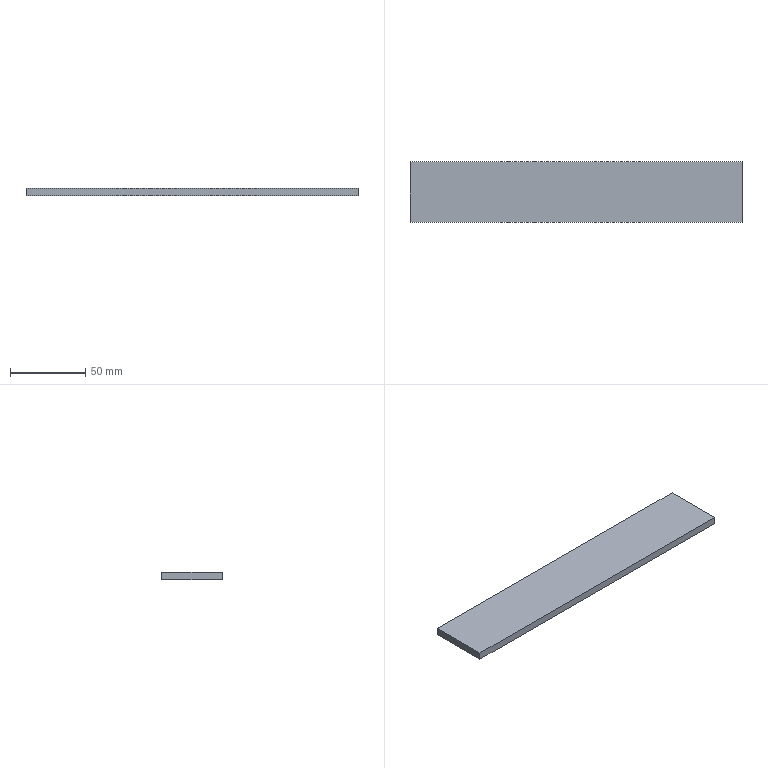Part | SolidWorks | features BaseBody 1 | 1 solid | 6 faces | box 220 x 40 x 5 mm | volume 44000 mm3 | plane 6
STEP:
#1=CARTESIAN_POINT('',(110.,-20.,0.));
#2=VERTEX_POINT('',#1);
#3=CARTESIAN_POINT('',(110.,20.,0.));
#4=VERTEX_POINT('',#3);
#5=CARTESIAN_POINT('',(110.,20.,0.));
#6=DIRECTION('',(0.,1.,0.));
#7=VECTOR('',#6,1000.);
#8=LINE('',#5,#7);
#9=EDGE_CURVE('',#2,#4,#8,.T.);
#10=ORIENTED_EDGE('',*,*,#9,.T.);
#11=CARTESIAN_POINT('',(-110.,20.,0.));
#12=VERTEX_POINT('',#11);
#13=CARTESIAN_POINT('',(-110.,20.,0.));
#14=DIRECTION('',(-1.,0.,0.));
#15=VECTOR('',#14,1000.);
#16=LINE('',#13,#15);
#17=EDGE_CURVE('',#4,#12,#16,.T.);
#18=ORIENTED_EDGE('',*,*,#17,.T.);
#19=CARTESIAN_POINT('',(-110.,-20.,0.));
#20=VERTEX_POINT('',#19);
#21=CARTESIAN_POINT('',(-110.,20.,0.));
#22=DIRECTION('',(0.,-1.,0.));
#23=VECTOR('',#22,1000.);
#24=LINE('',#21,#23);
#25=EDGE_CURVE('',#12,#20,#24,.T.);
#26=ORIENTED_EDGE('',*,*,#25,.T.);
#27=CARTESIAN_POINT('',(-110.,-20.,0.));
#28=DIRECTION('',(1.,0.,0.));
#29=VECTOR('',#28,1000.);
#30=LINE('',#27,#29);
#31=EDGE_CURVE('',#20,#2,#30,.T.);
#32=ORIENTED_EDGE('',*,*,#31,.T.);
#33=EDGE_LOOP('',(#10,#18,#26,#32));
#34=FACE_OUTER_BOUND('',#33,.T.);
#35=CARTESIAN_POINT('',(0.,0.,0.));
#36=DIRECTION('',(0.,0.,1.));
#37=DIRECTION('',(1.,0.,0.));
#38=AXIS2_PLACEMENT_3D('',#35,#36,#37);
#39=PLANE('',#38);
#40=ADVANCED_FACE('',(#34),#39,.T.);
#41=CARTESIAN_POINT('',(110.,-20.,-5.));
#42=VERTEX_POINT('',#41);
#43=CARTESIAN_POINT('',(110.,20.,-5.));
#44=VERTEX_POINT('',#43);
#45=CARTESIAN_POINT('',(110.,20.,-5.));
#46=DIRECTION('',(0.,1.,0.));
#47=VECTOR('',#46,1000.);
#48=LINE('',#45,#47);
#49=EDGE_CURVE('',#42,#44,#48,.T.);
#50=ORIENTED_EDGE('',*,*,#49,.F.);
#51=CARTESIAN_POINT('',(-110.,-20.,-5.));
#52=VERTEX_POINT('',#51);
#53=CARTESIAN_POINT('',(-110.,-20.,-5.));
#54=DIRECTION('',(1.,0.,0.));
#55=VECTOR('',#54,1000.);
#56=LINE('',#53,#55);
#57=EDGE_CURVE('',#52,#42,#56,.T.);
#58=ORIENTED_EDGE('',*,*,#57,.F.);
#59=CARTESIAN_POINT('',(-110.,20.,-5.));
#60=VERTEX_POINT('',#59);
#61=CARTESIAN_POINT('',(-110.,20.,-5.));
#62=DIRECTION('',(0.,-1.,0.));
#63=VECTOR('',#62,1000.);
#64=LINE('',#61,#63);
#65=EDGE_CURVE('',#60,#52,#64,.T.);
#66=ORIENTED_EDGE('',*,*,#65,.F.);
#67=CARTESIAN_POINT('',(-110.,20.,-5.));
#68=DIRECTION('',(-1.,0.,0.));
#69=VECTOR('',#68,1000.);
#70=LINE('',#67,#69);
#71=EDGE_CURVE('',#44,#60,#70,.T.);
#72=ORIENTED_EDGE('',*,*,#71,.F.);
#73=EDGE_LOOP('',(#50,#58,#66,#72));
#74=FACE_OUTER_BOUND('',#73,.T.);
#75=CARTESIAN_POINT('',(0.,0.,-5.));
#76=DIRECTION('',(0.,0.,1.));
#77=DIRECTION('',(1.,0.,0.));
#78=AXIS2_PLACEMENT_3D('',#75,#76,#77);
#79=PLANE('',#78);
#80=ADVANCED_FACE('',(#74),#79,.F.);
#81=ORIENTED_EDGE('',*,*,#17,.F.);
#82=CARTESIAN_POINT('',(110.,20.,-5.));
#83=DIRECTION('',(0.,0.,1.));
#84=VECTOR('',#83,1000.);
#85=LINE('',#82,#84);
#86=EDGE_CURVE('',#44,#4,#85,.T.);
#87=ORIENTED_EDGE('',*,*,#86,.F.);
#88=ORIENTED_EDGE('',*,*,#71,.T.);
#89=CARTESIAN_POINT('',(-110.,20.,-5.));
#90=DIRECTION('',(0.,0.,1.));
#91=VECTOR('',#90,1000.);
#92=LINE('',#89,#91);
#93=EDGE_CURVE('',#60,#12,#92,.T.);
#94=ORIENTED_EDGE('',*,*,#93,.T.);
#95=EDGE_LOOP('',(#81,#87,#88,#94));
#96=FACE_OUTER_BOUND('',#95,.T.);
#97=CARTESIAN_POINT('',(-110.,20.,-5.));
#98=DIRECTION('',(0.,1.,0.));
#99=DIRECTION('',(1.,0.,0.));
#100=AXIS2_PLACEMENT_3D('',#97,#98,#99);
#101=PLANE('',#100);
#102=ADVANCED_FACE('',(#96),#101,.T.);
#103=ORIENTED_EDGE('',*,*,#25,.F.);
#104=ORIENTED_EDGE('',*,*,#93,.F.);
#105=ORIENTED_EDGE('',*,*,#65,.T.);
#106=CARTESIAN_POINT('',(-110.,-20.,-5.));
#107=DIRECTION('',(0.,0.,1.));
#108=VECTOR('',#107,1000.);
#109=LINE('',#106,#108);
#110=EDGE_CURVE('',#52,#20,#109,.T.);
#111=ORIENTED_EDGE('',*,*,#110,.T.);
#112=EDGE_LOOP('',(#103,#104,#105,#111));
#113=FACE_OUTER_BOUND('',#112,.T.);
#114=CARTESIAN_POINT('',(-110.,20.,-5.));
#115=DIRECTION('',(-1.,0.,0.));
#116=DIRECTION('',(0.,0.,1.));
#117=AXIS2_PLACEMENT_3D('',#114,#115,#116);
#118=PLANE('',#117);
#119=ADVANCED_FACE('',(#113),#118,.T.);
#120=ORIENTED_EDGE('',*,*,#31,.F.);
#121=ORIENTED_EDGE('',*,*,#110,.F.);
#122=ORIENTED_EDGE('',*,*,#57,.T.);
#123=CARTESIAN_POINT('',(110.,-20.,-5.));
#124=DIRECTION('',(0.,0.,1.));
#125=VECTOR('',#124,1000.);
#126=LINE('',#123,#125);
#127=EDGE_CURVE('',#42,#2,#126,.T.);
#128=ORIENTED_EDGE('',*,*,#127,.T.);
#129=EDGE_LOOP('',(#120,#121,#122,#128));
#130=FACE_OUTER_BOUND('',#129,.T.);
#131=CARTESIAN_POINT('',(-110.,-20.,-5.));
#132=DIRECTION('',(0.,-1.,0.));
#133=DIRECTION('',(0.,0.,-1.));
#134=AXIS2_PLACEMENT_3D('',#131,#132,#133);
#135=PLANE('',#134);
#136=ADVANCED_FACE('',(#130),#135,.T.);
#137=ORIENTED_EDGE('',*,*,#9,.F.);
#138=ORIENTED_EDGE('',*,*,#127,.F.);
#139=ORIENTED_EDGE('',*,*,#49,.T.);
#140=ORIENTED_EDGE('',*,*,#86,.T.);
#141=EDGE_LOOP('',(#137,#138,#139,#140));
#142=FACE_OUTER_BOUND('',#141,.T.);
#143=CARTESIAN_POINT('',(110.,20.,-5.));
#144=DIRECTION('',(1.,0.,0.));
#145=DIRECTION('',(0.,1.,0.));
#146=AXIS2_PLACEMENT_3D('',#143,#144,#145);
#147=PLANE('',#146);
#148=ADVANCED_FACE('',(#142),#147,.T.);
#149=CLOSED_SHELL('',(#40,#80,#102,#119,#136,#148));
#150=MANIFOLD_SOLID_BREP('',#149);
#151=CARTESIAN_POINT('',(0.,0.,0.));
#152=DIRECTION('',(0.,0.,1.));
#153=DIRECTION('',(1.,0.,0.));
#154=AXIS2_PLACEMENT_3D('',#151,#152,#153);
#155=(LENGTH_UNIT()NAMED_UNIT(*)SI_UNIT(.MILLI.,.METRE.));
#156=UNCERTAINTY_MEASURE_WITH_UNIT(LENGTH_MEASURE(0.00001),#155,'','');
#157=(NAMED_UNIT(*)PLANE_ANGLE_UNIT()SI_UNIT($,.RADIAN.));
#158=(NAMED_UNIT(*)SI_UNIT($,.STERADIAN.)SOLID_ANGLE_UNIT());
#159=(GEOMETRIC_REPRESENTATION_CONTEXT(3)GLOBAL_UNCERTAINTY_ASSIGNED_CONTEXT((#156))GLOBAL_UNIT_ASSIGNED_CONTEXT((#155,#157,#158))REPRESENTATION_CONTEXT('',''));
#160=ADVANCED_BREP_SHAPE_REPRESENTATION('',(#150,#154),#159);